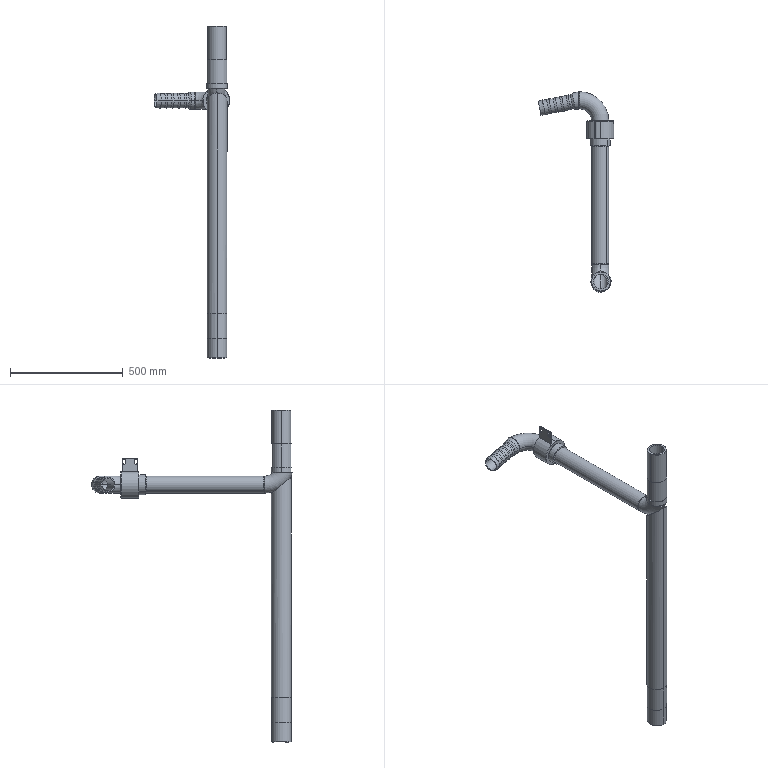Part | SolidWorks | features CompositeCurve 45, InContextFeatHolder 1 | 12 solids | 195 faces | box 335.143 x 891.073 x 1473 mm | volume 5779817 mm3 | cylinder 76 | cone 48 | plane 47 | torus 18 | spline 6 | commonest cylinder face diameters 85 x16 64 x10 89 x10 65 x8 13 x6 76 x6